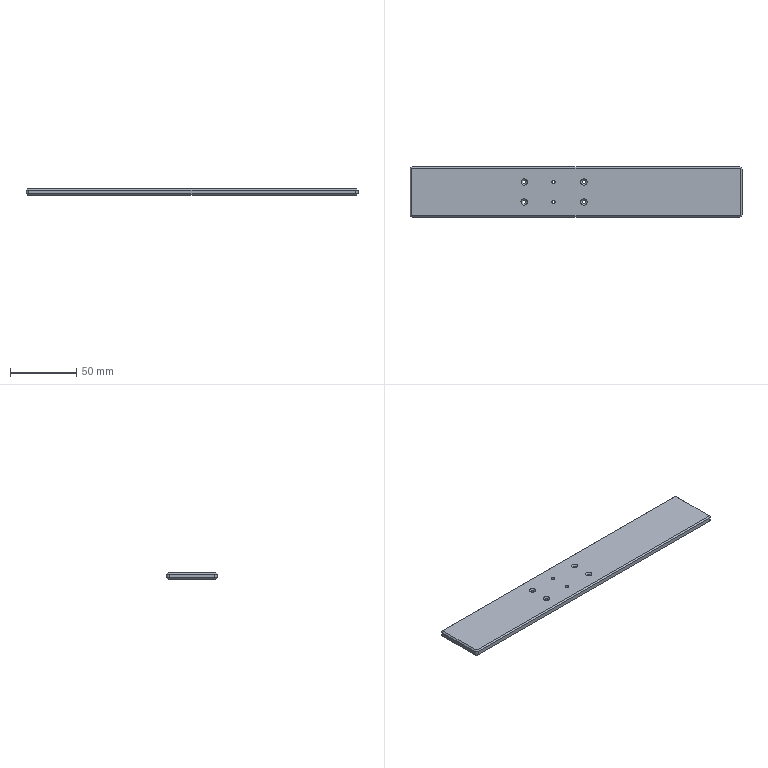NC program | NX | posted with a generic post | part box 250 x 38 x 5 mm
Lines 15278 to 15324 of 15324:
(ZLEVEL_PROFILE_COPY_1_COPY_COPY_COPY_COPY_COPY_COPY , TOOL : D6A45)
N30548 T09 M6
N30550 G54
N30552 G17 G0 G90 X-123.973 Y21.086 S7000 M3
N30554 G43 Z35. H9
N30556 Z3.
N30558 G94 G1 X-123.52 Y20.3 F1000.
N30560 G3 X-123. Y20. R0.6
N30562 G1 X123.
N30564 G2 X126. Y17. R3.
N30566 G1 Y-17.
N30568 G2 X123. Y-20. R3.
N30570 G1 X-123.
N30572 G2 X-126. Y-17. R3.
N30574 G1 Y17.
N30576 G2 X-123. Y20. R3.
N30578 G3 X-122.48 Y20.3 R0.6
N30580 G1 X-121.961 Y21.2
N30582 G0 Z35.
N30584 M5
(ZLEVEL_PROFILE_COPY_COPY_1_COPY , TOOL : D4)
N30586 T06 M6
N30588 G54
N30590 G17 G0 G90 X-123.8 Y21.733 S6000 M3
N30592 G43 Z35. H6
N30594 Z1.65
N30596 G94 G1 Z0.15 F1000.
N30598 X-123.788 Y21.661
N30600 G3 X-123. Y21. R0.8
N30602 G1 X123.
N30604 G2 X127. Y17. R4.
N30606 G1 Y-17.
N30608 G2 X123. Y-21. R4.
N30610 G1 X-123.
N30612 G2 X-127. Y-17. R4.
N30614 G1 Y17.
N30616 G2 X-123. Y21. R4.
N30618 G3 X-122.212 Y21.661 R0.8
N30620 G1 X-122.188 Y21.8
N30622 Z1.65
N30624 G0 Z35.
N30626 M5
N30628 M2